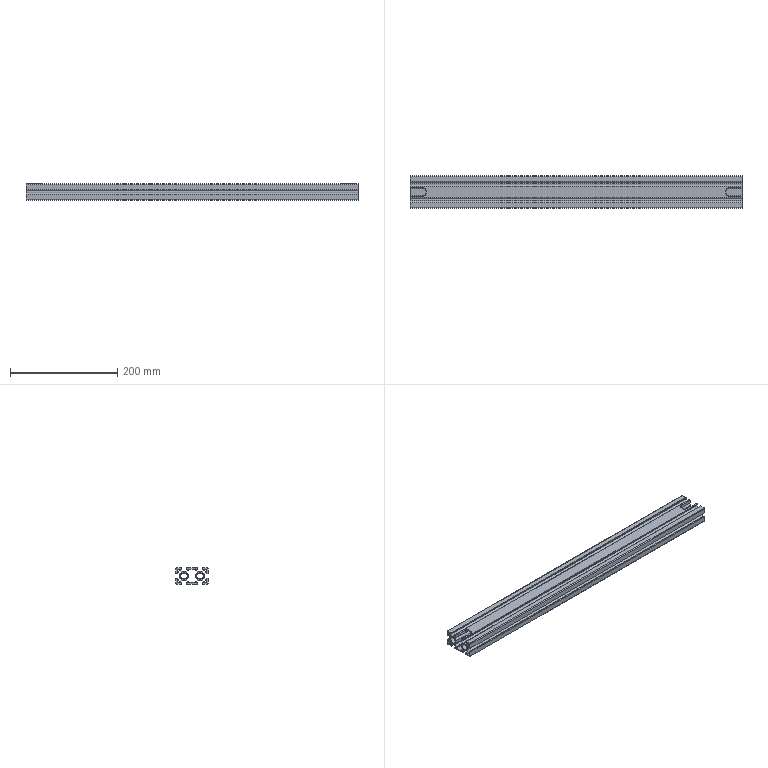Part | STEP file | belt line support ET profile 620 | 1 solid | 174 faces | box 620 x 60 x 30 mm | volume 399085 mm3 | plane 92 | cylinder 74 | cone 8 | commonest cylinder face diameters 2 x26 16 x14 1 x10 10 x8 12 x8 3 x4